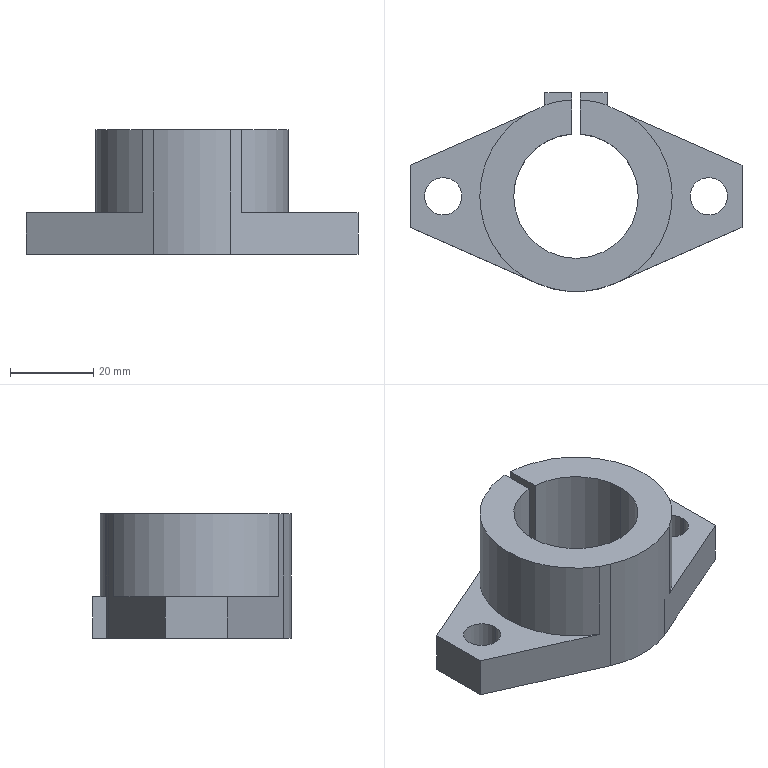Part | STEP file | SHF30 | 1 solid | 33 faces | box 80 x 48 x 30 mm | volume 36862 mm3 | plane 18 | cylinder 15 | commonest cylinder face diameters 46.376 x5 9 x4 30 x3 46 x3